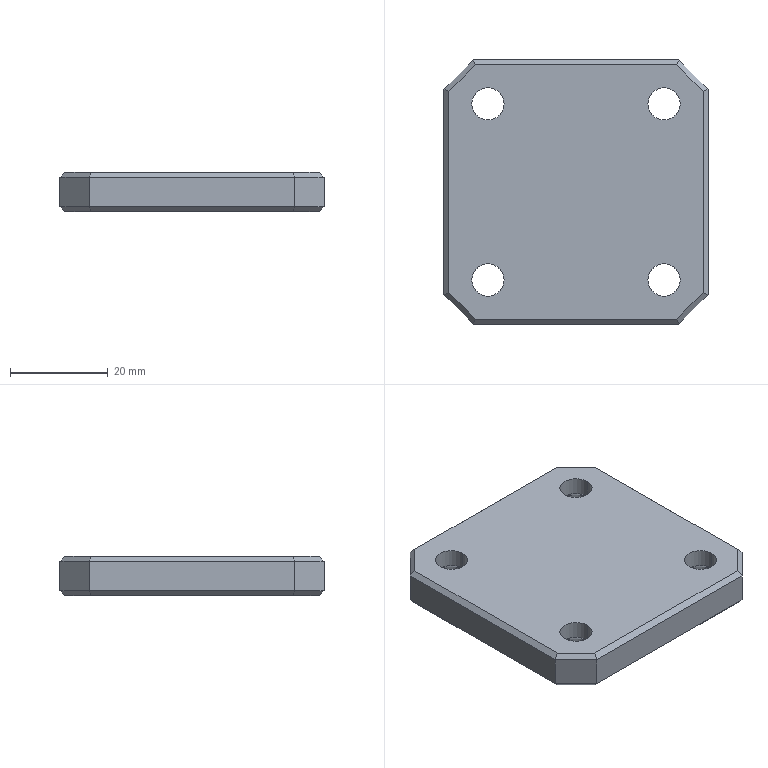Part | Creo | 1 solid | 50 faces | box 54 x 53.991 x 8 mm | volume 20318 mm3 | plane 26 | cylinder 16 | cone 8 | commonest cylinder face diameters 6.6 x8 13 x8
STEP:
#1=CARTESIAN_POINT('',(-106.,282.581,-2.));
#2=VERTEX_POINT('',#1);
#3=CARTESIAN_POINT('',(-106.,241.419,-2.));
#4=VERTEX_POINT('',#3);
#5=CARTESIAN_POINT('',(-106.,282.581,-2.));
#6=DIRECTION('',(0.,-1.,0.));
#7=VECTOR('',#6,41.162);
#8=LINE('',#5,#7);
#9=EDGE_CURVE('',#2,#4,#8,.T.);
#10=ORIENTED_EDGE('',*,*,#9,.T.);
#11=CARTESIAN_POINT('',(-111.414,236.005,-2.));
#12=VERTEX_POINT('',#11);
#13=CARTESIAN_POINT('',(-111.414,236.005,-2.));
#14=DIRECTION('',(0.7071,0.7071,0.));
#15=VECTOR('',#14,7.657);
#16=LINE('',#13,#15);
#17=EDGE_CURVE('',#12,#4,#16,.T.);
#18=ORIENTED_EDGE('',*,*,#17,.F.);
#19=CARTESIAN_POINT('',(-152.586,236.005,-2.));
#20=VERTEX_POINT('',#19);
#21=CARTESIAN_POINT('',(-111.414,236.005,-2.));
#22=DIRECTION('',(-1.,0.,0.));
#23=VECTOR('',#22,41.172);
#24=LINE('',#21,#23);
#25=EDGE_CURVE('',#12,#20,#24,.T.);
#26=ORIENTED_EDGE('',*,*,#25,.T.);
#27=CARTESIAN_POINT('',(-158.,241.419,-2.));
#28=VERTEX_POINT('',#27);
#29=CARTESIAN_POINT('',(-158.,241.419,-2.));
#30=DIRECTION('',(0.7071,-0.7071,0.));
#31=VECTOR('',#30,7.657);
#32=LINE('',#29,#31);
#33=EDGE_CURVE('',#28,#20,#32,.T.);
#34=ORIENTED_EDGE('',*,*,#33,.F.);
#35=CARTESIAN_POINT('',(-158.,282.581,-2.));
#36=VERTEX_POINT('',#35);
#37=CARTESIAN_POINT('',(-158.,241.419,-2.));
#38=DIRECTION('',(0.,1.,0.));
#39=VECTOR('',#38,41.162);
#40=LINE('',#37,#39);
#41=EDGE_CURVE('',#28,#36,#40,.T.);
#42=ORIENTED_EDGE('',*,*,#41,.T.);
#43=CARTESIAN_POINT('',(-152.586,287.995,-2.));
#44=VERTEX_POINT('',#43);
#45=CARTESIAN_POINT('',(-152.586,287.995,-2.));
#46=DIRECTION('',(-0.7071,-0.7071,0.));
#47=VECTOR('',#46,7.657);
#48=LINE('',#45,#47);
#49=EDGE_CURVE('',#44,#36,#48,.T.);
#50=ORIENTED_EDGE('',*,*,#49,.F.);
#51=CARTESIAN_POINT('',(-111.414,287.995,-2.));
#52=VERTEX_POINT('',#51);
#53=CARTESIAN_POINT('',(-152.586,287.995,-2.));
#54=DIRECTION('',(1.,0.,0.));
#55=VECTOR('',#54,41.172);
#56=LINE('',#53,#55);
#57=EDGE_CURVE('',#44,#52,#56,.T.);
#58=ORIENTED_EDGE('',*,*,#57,.T.);
#59=CARTESIAN_POINT('',(-106.,282.581,-2.));
#60=DIRECTION('',(-0.7071,0.7071,0.));
#61=VECTOR('',#60,7.657);
#62=LINE('',#59,#61);
#63=EDGE_CURVE('',#2,#52,#62,.T.);
#64=ORIENTED_EDGE('',*,*,#63,.F.);
#65=EDGE_LOOP('',(#10,#18,#26,#34,#42,#50,#58,#64));
#66=FACE_OUTER_BOUND('',#65,.F.);
#67=CARTESIAN_POINT('',(-110.7,280.005,-2.));
#68=VERTEX_POINT('',#67);
#69=CARTESIAN_POINT('',(-117.3,280.005,-2.));
#70=VERTEX_POINT('',#69);
#71=CARTESIAN_POINT('',(-114.,280.005,-2.));
#72=DIRECTION('',(0.,0.,-1.));
#73=DIRECTION('',(1.,0.,0.));
#74=AXIS2_PLACEMENT_3D('',#71,#72,#73);
#75=CIRCLE('',#74,3.3);
#76=EDGE_CURVE('',#68,#70,#75,.T.);
#77=ORIENTED_EDGE('',*,*,#76,.F.);
#78=CARTESIAN_POINT('',(-114.,280.005,-2.));
#79=DIRECTION('',(0.,0.,-1.));
#80=DIRECTION('',(-1.,0.,0.));
#81=AXIS2_PLACEMENT_3D('',#78,#79,#80);
#82=CIRCLE('',#81,3.3);
#83=EDGE_CURVE('',#70,#68,#82,.T.);
#84=ORIENTED_EDGE('',*,*,#83,.F.);
#85=EDGE_LOOP('',(#77,#84));
#86=FACE_BOUND('',#85,.F.);
#87=CARTESIAN_POINT('',(-146.7,280.005,-2.));
#88=VERTEX_POINT('',#87);
#89=CARTESIAN_POINT('',(-153.3,280.005,-2.));
#90=VERTEX_POINT('',#89);
#91=CARTESIAN_POINT('',(-150.,280.005,-2.));
#92=DIRECTION('',(0.,0.,-1.));
#93=DIRECTION('',(1.,0.,0.));
#94=AXIS2_PLACEMENT_3D('',#91,#92,#93);
#95=CIRCLE('',#94,3.3);
#96=EDGE_CURVE('',#88,#90,#95,.T.);
#97=ORIENTED_EDGE('',*,*,#96,.F.);
#98=CARTESIAN_POINT('',(-150.,280.005,-2.));
#99=DIRECTION('',(0.,0.,-1.));
#100=DIRECTION('',(-1.,0.,0.));
#101=AXIS2_PLACEMENT_3D('',#98,#99,#100);
#102=CIRCLE('',#101,3.3);
#103=EDGE_CURVE('',#90,#88,#102,.T.);
#104=ORIENTED_EDGE('',*,*,#103,.F.);
#105=EDGE_LOOP('',(#97,#104));
#106=FACE_BOUND('',#105,.F.);
#107=CARTESIAN_POINT('',(-110.7,244.005,-2.));
#108=VERTEX_POINT('',#107);
#109=CARTESIAN_POINT('',(-117.3,244.005,-2.));
#110=VERTEX_POINT('',#109);
#111=CARTESIAN_POINT('',(-114.,244.005,-2.));
#112=DIRECTION('',(0.,0.,-1.));
#113=DIRECTION('',(1.,0.,0.));
#114=AXIS2_PLACEMENT_3D('',#111,#112,#113);
#115=CIRCLE('',#114,3.3);
#116=EDGE_CURVE('',#108,#110,#115,.T.);
#117=ORIENTED_EDGE('',*,*,#116,.F.);
#118=CARTESIAN_POINT('',(-114.,244.005,-2.));
#119=DIRECTION('',(0.,0.,-1.));
#120=DIRECTION('',(-1.,0.,0.));
#121=AXIS2_PLACEMENT_3D('',#118,#119,#120);
#122=CIRCLE('',#121,3.3);
#123=EDGE_CURVE('',#110,#108,#122,.T.);
#124=ORIENTED_EDGE('',*,*,#123,.F.);
#125=EDGE_LOOP('',(#117,#124));
#126=FACE_BOUND('',#125,.F.);
#127=CARTESIAN_POINT('',(-146.7,244.005,-2.));
#128=VERTEX_POINT('',#127);
#129=CARTESIAN_POINT('',(-153.3,244.005,-2.));
#130=VERTEX_POINT('',#129);
#131=CARTESIAN_POINT('',(-150.,244.005,-2.));
#132=DIRECTION('',(0.,0.,-1.));
#133=DIRECTION('',(1.,0.,0.));
#134=AXIS2_PLACEMENT_3D('',#131,#132,#133);
#135=CIRCLE('',#134,3.3);
#136=EDGE_CURVE('',#128,#130,#135,.T.);
#137=ORIENTED_EDGE('',*,*,#136,.F.);
#138=CARTESIAN_POINT('',(-150.,244.005,-2.));
#139=DIRECTION('',(0.,0.,-1.));
#140=DIRECTION('',(-1.,0.,0.));
#141=AXIS2_PLACEMENT_3D('',#138,#139,#140);
#142=CIRCLE('',#141,3.3);
#143=EDGE_CURVE('',#130,#128,#142,.T.);
#144=ORIENTED_EDGE('',*,*,#143,.F.);
#145=EDGE_LOOP('',(#137,#144));
#146=FACE_BOUND('',#145,.F.);
#147=CARTESIAN_POINT('',(-132.,262.005,-2.));
#148=DIRECTION('',(0.,0.,1.));
#149=DIRECTION('',(-1.,0.,0.));
#150=AXIS2_PLACEMENT_3D('',#147,#148,#149);
#151=PLANE('',#150);
#152=ADVANCED_FACE('',(#66,#86,#106,#126,#146),#151,.T.);
#153=CARTESIAN_POINT('',(-105.,282.995,-3.));
#154=VERTEX_POINT('',#153);
#155=CARTESIAN_POINT('',(-106.,282.581,-2.));
#156=DIRECTION('',(0.6786,0.2811,-0.6786));
#157=VECTOR('',#156,1.474);
#158=LINE('',#155,#157);
#159=EDGE_CURVE('',#2,#154,#158,.T.);
#160=ORIENTED_EDGE('',*,*,#159,.T.);
#161=CARTESIAN_POINT('',(-105.,241.005,-3.));
#162=VERTEX_POINT('',#161);
#163=CARTESIAN_POINT('',(-105.,241.005,-3.));
#164=DIRECTION('',(0.,1.,0.));
#165=VECTOR('',#164,41.991);
#166=LINE('',#163,#165);
#167=EDGE_CURVE('',#162,#154,#166,.T.);
#168=ORIENTED_EDGE('',*,*,#167,.F.);
#169=CARTESIAN_POINT('',(-106.,241.419,-2.));
#170=DIRECTION('',(0.6786,-0.2811,-0.6786));
#171=VECTOR('',#170,1.474);
#172=LINE('',#169,#171);
#173=EDGE_CURVE('',#4,#162,#172,.T.);
#174=ORIENTED_EDGE('',*,*,#173,.F.);
#175=ORIENTED_EDGE('',*,*,#9,.F.);
#176=EDGE_LOOP('',(#160,#168,#174,#175));
#177=FACE_OUTER_BOUND('',#176,.F.);
#178=CARTESIAN_POINT('',(-105.,262.005,-3.));
#179=DIRECTION('',(-0.7071,0.,-0.7071));
#180=DIRECTION('',(0.,-1.,0.));
#181=AXIS2_PLACEMENT_3D('',#178,#179,#180);
#182=PLANE('',#181);
#183=ADVANCED_FACE('',(#177),#182,.F.);
#184=CARTESIAN_POINT('',(-111.,288.995,-3.));
#185=VERTEX_POINT('',#184);
#186=CARTESIAN_POINT('',(-111.414,287.995,-2.));
#187=DIRECTION('',(0.2811,0.6786,-0.6786));
#188=VECTOR('',#187,1.474);
#189=LINE('',#186,#188);
#190=EDGE_CURVE('',#52,#185,#189,.T.);
#191=ORIENTED_EDGE('',*,*,#190,.T.);
#192=CARTESIAN_POINT('',(-105.,282.995,-3.));
#193=DIRECTION('',(-0.7071,0.7071,0.));
#194=VECTOR('',#193,8.485);
#195=LINE('',#192,#194);
#196=EDGE_CURVE('',#154,#185,#195,.T.);
#197=ORIENTED_EDGE('',*,*,#196,.F.);
#198=ORIENTED_EDGE('',*,*,#159,.F.);
#199=ORIENTED_EDGE('',*,*,#63,.T.);
#200=EDGE_LOOP('',(#191,#197,#198,#199));
#201=FACE_OUTER_BOUND('',#200,.F.);
#202=CARTESIAN_POINT('',(-108.712,285.293,-2.));
#203=DIRECTION('',(0.5,0.5,0.7071));
#204=DIRECTION('',(0.7071,-0.7071,0.));
#205=AXIS2_PLACEMENT_3D('',#202,#203,#204);
#206=PLANE('',#205);
#207=ADVANCED_FACE('',(#201),#206,.T.);
#208=CARTESIAN_POINT('',(-153.,288.995,-3.));
#209=VERTEX_POINT('',#208);
#210=CARTESIAN_POINT('',(-153.,288.995,-3.));
#211=DIRECTION('',(0.2811,-0.6786,0.6786));
#212=VECTOR('',#211,1.474);
#213=LINE('',#210,#212);
#214=EDGE_CURVE('',#209,#44,#213,.T.);
#215=ORIENTED_EDGE('',*,*,#214,.F.);
#216=CARTESIAN_POINT('',(-111.,288.995,-3.));
#217=DIRECTION('',(-1.,0.,0.));
#218=VECTOR('',#217,42.);
#219=LINE('',#216,#218);
#220=EDGE_CURVE('',#185,#209,#219,.T.);
#221=ORIENTED_EDGE('',*,*,#220,.F.);
#222=ORIENTED_EDGE('',*,*,#190,.F.);
#223=ORIENTED_EDGE('',*,*,#57,.F.);
#224=EDGE_LOOP('',(#215,#221,#222,#223));
#225=FACE_OUTER_BOUND('',#224,.F.);
#226=CARTESIAN_POINT('',(-132.,288.995,-3.));
#227=DIRECTION('',(0.,-0.7071,-0.7071));
#228=DIRECTION('',(1.,0.,0.));
#229=AXIS2_PLACEMENT_3D('',#226,#227,#228);
#230=PLANE('',#229);
#231=ADVANCED_FACE('',(#225),#230,.F.);
#232=ORIENTED_EDGE('',*,*,#214,.T.);
#233=ORIENTED_EDGE('',*,*,#49,.T.);
#234=CARTESIAN_POINT('',(-159.,282.995,-3.));
#235=VERTEX_POINT('',#234);
#236=CARTESIAN_POINT('',(-159.,282.995,-3.));
#237=DIRECTION('',(0.6786,-0.2811,0.6786));
#238=VECTOR('',#237,1.474);
#239=LINE('',#236,#238);
#240=EDGE_CURVE('',#235,#36,#239,.T.);
#241=ORIENTED_EDGE('',*,*,#240,.F.);
#242=CARTESIAN_POINT('',(-153.,288.995,-3.));
#243=DIRECTION('',(-0.7071,-0.7071,0.));
#244=VECTOR('',#243,8.485);
#245=LINE('',#242,#244);
#246=EDGE_CURVE('',#209,#235,#245,.T.);
#247=ORIENTED_EDGE('',*,*,#246,.F.);
#248=EDGE_LOOP('',(#232,#233,#241,#247));
#249=FACE_OUTER_BOUND('',#248,.F.);
#250=CARTESIAN_POINT('',(-155.288,285.293,-2.));
#251=DIRECTION('',(-0.5,0.5,0.7071));
#252=DIRECTION('',(0.7071,0.7071,0.));
#253=AXIS2_PLACEMENT_3D('',#250,#251,#252);
#254=PLANE('',#253);
#255=ADVANCED_FACE('',(#249),#254,.T.);
#256=ORIENTED_EDGE('',*,*,#240,.T.);
#257=ORIENTED_EDGE('',*,*,#41,.F.);
#258=CARTESIAN_POINT('',(-159.,241.005,-3.));
#259=VERTEX_POINT('',#258);
#260=CARTESIAN_POINT('',(-159.,241.005,-3.));
#261=DIRECTION('',(0.6786,0.2811,0.6786));
#262=VECTOR('',#261,1.474);
#263=LINE('',#260,#262);
#264=EDGE_CURVE('',#259,#28,#263,.T.);
#265=ORIENTED_EDGE('',*,*,#264,.F.);
#266=CARTESIAN_POINT('',(-159.,282.995,-3.));
#267=DIRECTION('',(0.,-1.,0.));
#268=VECTOR('',#267,41.991);
#269=LINE('',#266,#268);
#270=EDGE_CURVE('',#235,#259,#269,.T.);
#271=ORIENTED_EDGE('',*,*,#270,.F.);
#272=EDGE_LOOP('',(#256,#257,#265,#271));
#273=FACE_OUTER_BOUND('',#272,.F.);
#274=CARTESIAN_POINT('',(-159.,262.005,-3.));
#275=DIRECTION('',(0.7071,0.,-0.7071));
#276=DIRECTION('',(0.,1.,0.));
#277=AXIS2_PLACEMENT_3D('',#274,#275,#276);
#278=PLANE('',#277);
#279=ADVANCED_FACE('',(#273),#278,.F.);
#280=ORIENTED_EDGE('',*,*,#264,.T.);
#281=ORIENTED_EDGE('',*,*,#33,.T.);
#282=CARTESIAN_POINT('',(-153.,235.005,-3.));
#283=VERTEX_POINT('',#282);
#284=CARTESIAN_POINT('',(-153.,235.005,-3.));
#285=DIRECTION('',(0.2811,0.6786,0.6786));
#286=VECTOR('',#285,1.474);
#287=LINE('',#284,#286);
#288=EDGE_CURVE('',#283,#20,#287,.T.);
#289=ORIENTED_EDGE('',*,*,#288,.F.);
#290=CARTESIAN_POINT('',(-159.,241.005,-3.));
#291=DIRECTION('',(0.7071,-0.7071,0.));
#292=VECTOR('',#291,8.485);
#293=LINE('',#290,#292);
#294=EDGE_CURVE('',#259,#283,#293,.T.);
#295=ORIENTED_EDGE('',*,*,#294,.F.);
#296=EDGE_LOOP('',(#280,#281,#289,#295));
#297=FACE_OUTER_BOUND('',#296,.F.);
#298=CARTESIAN_POINT('',(-155.293,238.712,-2.));
#299=DIRECTION('',(-0.5,-0.5,0.7071));
#300=DIRECTION('',(-0.7071,0.7071,0.));
#301=AXIS2_PLACEMENT_3D('',#298,#299,#300);
#302=PLANE('',#301);
#303=ADVANCED_FACE('',(#297),#302,.T.);
#304=CARTESIAN_POINT('',(-111.,235.005,-3.));
#305=VERTEX_POINT('',#304);
#306=CARTESIAN_POINT('',(-111.414,236.005,-2.));
#307=DIRECTION('',(0.2811,-0.6786,-0.6786));
#308=VECTOR('',#307,1.474);
#309=LINE('',#306,#308);
#310=EDGE_CURVE('',#12,#305,#309,.T.);
#311=ORIENTED_EDGE('',*,*,#310,.T.);
#312=CARTESIAN_POINT('',(-153.,235.005,-3.));
#313=DIRECTION('',(1.,0.,0.));
#314=VECTOR('',#313,42.);
#315=LINE('',#312,#314);
#316=EDGE_CURVE('',#283,#305,#315,.T.);
#317=ORIENTED_EDGE('',*,*,#316,.F.);
#318=ORIENTED_EDGE('',*,*,#288,.T.);
#319=ORIENTED_EDGE('',*,*,#25,.F.);
#320=EDGE_LOOP('',(#311,#317,#318,#319));
#321=FACE_OUTER_BOUND('',#320,.F.);
#322=CARTESIAN_POINT('',(-132.,235.005,-3.));
#323=DIRECTION('',(0.,0.7071,-0.7071));
#324=DIRECTION('',(-1.,0.,0.));
#325=AXIS2_PLACEMENT_3D('',#322,#323,#324);
#326=PLANE('',#325);
#327=ADVANCED_FACE('',(#321),#326,.F.);
#328=ORIENTED_EDGE('',*,*,#173,.T.);
#329=CARTESIAN_POINT('',(-111.,235.005,-3.));
#330=DIRECTION('',(0.7071,0.7071,0.));
#331=VECTOR('',#330,8.485);
#332=LINE('',#329,#331);
#333=EDGE_CURVE('',#305,#162,#332,.T.);
#334=ORIENTED_EDGE('',*,*,#333,.F.);
#335=ORIENTED_EDGE('',*,*,#310,.F.);
#336=ORIENTED_EDGE('',*,*,#17,.T.);
#337=EDGE_LOOP('',(#328,#334,#335,#336));
#338=FACE_OUTER_BOUND('',#337,.F.);
#339=CARTESIAN_POINT('',(-108.707,238.712,-2.));
#340=DIRECTION('',(0.5,-0.5,0.7071));
#341=DIRECTION('',(-0.7071,-0.7071,0.));
#342=AXIS2_PLACEMENT_3D('',#339,#340,#341);
#343=PLANE('',#342);
#344=ADVANCED_FACE('',(#338),#343,.T.);
#345=CARTESIAN_POINT('',(-105.,241.005,-9.));
#346=VERTEX_POINT('',#345);
#347=CARTESIAN_POINT('',(-105.,241.005,-9.));
#348=DIRECTION('',(0.,0.,1.));
#349=VECTOR('',#348,6.);
#350=LINE('',#347,#349);
#351=EDGE_CURVE('',#346,#162,#350,.T.);
#352=ORIENTED_EDGE('',*,*,#351,.F.);
#353=CARTESIAN_POINT('',(-111.,235.005,-9.));
#354=VERTEX_POINT('',#353);
#355=CARTESIAN_POINT('',(-105.,241.005,-9.));
#356=DIRECTION('',(-0.7071,-0.7071,0.));
#357=VECTOR('',#356,8.485);
#358=LINE('',#355,#357);
#359=EDGE_CURVE('',#346,#354,#358,.T.);
#360=ORIENTED_EDGE('',*,*,#359,.T.);
#361=CARTESIAN_POINT('',(-111.,235.005,-3.));
#362=DIRECTION('',(0.,0.,-1.));
#363=VECTOR('',#362,6.);
#364=LINE('',#361,#363);
#365=EDGE_CURVE('',#305,#354,#364,.T.);
#366=ORIENTED_EDGE('',*,*,#365,.F.);
#367=ORIENTED_EDGE('',*,*,#333,.T.);
#368=EDGE_LOOP('',(#352,#360,#366,#367));
#369=FACE_OUTER_BOUND('',#368,.F.);
#370=CARTESIAN_POINT('',(-105.,241.005,-11.));
#371=DIRECTION('',(-0.7071,0.7071,0.));
#372=DIRECTION('',(0.,0.,-1.));
#373=AXIS2_PLACEMENT_3D('',#370,#371,#372);
#374=PLANE('',#373);
#375=ADVANCED_FACE('',(#369),#374,.F.);
#376=ORIENTED_EDGE('',*,*,#351,.T.);
#377=ORIENTED_EDGE('',*,*,#167,.T.);
#378=CARTESIAN_POINT('',(-105.,282.995,-9.));
#379=VERTEX_POINT('',#378);
#380=CARTESIAN_POINT('',(-105.,282.995,-3.));
#381=DIRECTION('',(0.,0.,-1.));
#382=VECTOR('',#381,6.);
#383=LINE('',#380,#382);
#384=EDGE_CURVE('',#154,#379,#383,.T.);
#385=ORIENTED_EDGE('',*,*,#384,.T.);
#386=CARTESIAN_POINT('',(-105.,282.995,-9.));
#387=DIRECTION('',(0.,-1.,0.));
#388=VECTOR('',#387,41.991);
#389=LINE('',#386,#388);
#390=EDGE_CURVE('',#379,#346,#389,.T.);
#391=ORIENTED_EDGE('',*,*,#390,.T.);
#392=EDGE_LOOP('',(#376,#377,#385,#391));
#393=FACE_OUTER_BOUND('',#392,.F.);
#394=CARTESIAN_POINT('',(-105.,262.005,-11.));
#395=DIRECTION('',(1.,0.,0.));
#396=DIRECTION('',(0.,0.,1.));
#397=AXIS2_PLACEMENT_3D('',#394,#395,#396);
#398=PLANE('',#397);
#399=ADVANCED_FACE('',(#393),#398,.T.);
#400=CARTESIAN_POINT('',(-111.,288.995,-9.));
#401=VERTEX_POINT('',#400);
#402=CARTESIAN_POINT('',(-111.,288.995,-9.));
#403=DIRECTION('',(0.,0.,1.));
#404=VECTOR('',#403,6.);
#405=LINE('',#402,#404);
#406=EDGE_CURVE('',#401,#185,#405,.T.);
#407=ORIENTED_EDGE('',*,*,#406,.F.);
#408=CARTESIAN_POINT('',(-111.,288.995,-9.));
#409=DIRECTION('',(0.7071,-0.7071,0.));
#410=VECTOR('',#409,8.485);
#411=LINE('',#408,#410);
#412=EDGE_CURVE('',#401,#379,#411,.T.);
#413=ORIENTED_EDGE('',*,*,#412,.T.);
#414=ORIENTED_EDGE('',*,*,#384,.F.);
#415=ORIENTED_EDGE('',*,*,#196,.T.);
#416=EDGE_LOOP('',(#407,#413,#414,#415));
#417=FACE_OUTER_BOUND('',#416,.F.);
#418=CARTESIAN_POINT('',(-111.,288.995,-10.));
#419=DIRECTION('',(-0.7071,-0.7071,0.));
#420=DIRECTION('',(0.,0.,-1.));
#421=AXIS2_PLACEMENT_3D('',#418,#419,#420);
#422=PLANE('',#421);
#423=ADVANCED_FACE('',(#417),#422,.F.);
#424=CARTESIAN_POINT('',(-153.,288.995,-9.));
#425=VERTEX_POINT('',#424);
#426=CARTESIAN_POINT('',(-153.,288.995,-3.));
#427=DIRECTION('',(0.,0.,-1.));
#428=VECTOR('',#427,6.);
#429=LINE('',#426,#428);
#430=EDGE_CURVE('',#209,#425,#429,.T.);
#431=ORIENTED_EDGE('',*,*,#430,.T.);
#432=CARTESIAN_POINT('',(-153.,288.995,-9.));
#433=DIRECTION('',(1.,0.,0.));
#434=VECTOR('',#433,42.);
#435=LINE('',#432,#434);
#436=EDGE_CURVE('',#425,#401,#435,.T.);
#437=ORIENTED_EDGE('',*,*,#436,.T.);
#438=ORIENTED_EDGE('',*,*,#406,.T.);
#439=ORIENTED_EDGE('',*,*,#220,.T.);
#440=EDGE_LOOP('',(#431,#437,#438,#439));
#441=FACE_OUTER_BOUND('',#440,.F.);
#442=CARTESIAN_POINT('',(-132.,288.995,-10.));
#443=DIRECTION('',(0.,1.,0.));
#444=DIRECTION('',(0.,0.,1.));
#445=AXIS2_PLACEMENT_3D('',#442,#443,#444);
#446=PLANE('',#445);
#447=ADVANCED_FACE('',(#441),#446,.T.);
#448=CARTESIAN_POINT('',(-159.,282.995,-9.));
#449=VERTEX_POINT('',#448);
#450=CARTESIAN_POINT('',(-159.,282.995,-9.));
#451=DIRECTION('',(0.,0.,1.));
#452=VECTOR('',#451,6.);
#453=LINE('',#450,#452);
#454=EDGE_CURVE('',#449,#235,#453,.T.);
#455=ORIENTED_EDGE('',*,*,#454,.F.);
#456=CARTESIAN_POINT('',(-159.,282.995,-9.));
#457=DIRECTION('',(0.7071,0.7071,0.));
#458=VECTOR('',#457,8.485);
#459=LINE('',#456,#458);
#460=EDGE_CURVE('',#449,#425,#459,.T.);
#461=ORIENTED_EDGE('',*,*,#460,.T.);
#462=ORIENTED_EDGE('',*,*,#430,.F.);
#463=ORIENTED_EDGE('',*,*,#246,.T.);
#464=EDGE_LOOP('',(#455,#461,#462,#463));
#465=FACE_OUTER_BOUND('',#464,.F.);
#466=CARTESIAN_POINT('',(-153.,288.995,-10.));
#467=DIRECTION('',(0.7071,-0.7071,0.));
#468=DIRECTION('',(0.,0.,1.));
#469=AXIS2_PLACEMENT_3D('',#466,#467,#468);
#470=PLANE('',#469);
#471=ADVANCED_FACE('',(#465),#470,.F.);
#472=ORIENTED_EDGE('',*,*,#454,.T.);
#473=ORIENTED_EDGE('',*,*,#270,.T.);
#474=CARTESIAN_POINT('',(-159.,241.005,-9.));
#475=VERTEX_POINT('',#474);
#476=CARTESIAN_POINT('',(-159.,241.005,-3.));
#477=DIRECTION('',(0.,0.,-1.));
#478=VECTOR('',#477,6.);
#479=LINE('',#476,#478);
#480=EDGE_CURVE('',#259,#475,#479,.T.);
#481=ORIENTED_EDGE('',*,*,#480,.T.);
#482=CARTESIAN_POINT('',(-159.,241.005,-9.));
#483=DIRECTION('',(0.,1.,0.));
#484=VECTOR('',#483,41.991);
#485=LINE('',#482,#484);
#486=EDGE_CURVE('',#475,#449,#485,.T.);
#487=ORIENTED_EDGE('',*,*,#486,.T.);
#488=EDGE_LOOP('',(#472,#473,#481,#487));
#489=FACE_OUTER_BOUND('',#488,.F.);
#490=CARTESIAN_POINT('',(-159.,262.005,-11.));
#491=DIRECTION('',(-1.,0.,0.));
#492=DIRECTION('',(0.,0.,-1.));
#493=AXIS2_PLACEMENT_3D('',#490,#491,#492);
#494=PLANE('',#493);
#495=ADVANCED_FACE('',(#489),#494,.T.);
#496=CARTESIAN_POINT('',(-153.,235.005,-9.));
#497=VERTEX_POINT('',#496);
#498=CARTESIAN_POINT('',(-153.,235.005,-9.));
#499=DIRECTION('',(0.,0.,1.));
#500=VECTOR('',#499,6.);
#501=LINE('',#498,#500);
#502=EDGE_CURVE('',#497,#283,#501,.T.);
#503=ORIENTED_EDGE('',*,*,#502,.F.);
#504=CARTESIAN_POINT('',(-153.,235.005,-9.));
#505=DIRECTION('',(-0.7071,0.7071,0.));
#506=VECTOR('',#505,8.485);
#507=LINE('',#504,#506);
#508=EDGE_CURVE('',#497,#475,#507,.T.);
#509=ORIENTED_EDGE('',*,*,#508,.T.);
#510=ORIENTED_EDGE('',*,*,#480,.F.);
#511=ORIENTED_EDGE('',*,*,#294,.T.);
#512=EDGE_LOOP('',(#503,#509,#510,#511));
#513=FACE_OUTER_BOUND('',#512,.F.);
#514=CARTESIAN_POINT('',(-159.,241.005,-11.));
#515=DIRECTION('',(0.7071,0.7071,0.));
#516=DIRECTION('',(0.,0.,1.));
#517=AXIS2_PLACEMENT_3D('',#514,#515,#516);
#518=PLANE('',#517);
#519=ADVANCED_FACE('',(#513),#518,.F.);
#520=ORIENTED_EDGE('',*,*,#502,.T.);
#521=ORIENTED_EDGE('',*,*,#316,.T.);
#522=ORIENTED_EDGE('',*,*,#365,.T.);
#523=CARTESIAN_POINT('',(-111.,235.005,-9.));
#524=DIRECTION('',(-1.,0.,0.));
#525=VECTOR('',#524,42.);
#526=LINE('',#523,#525);
#527=EDGE_CURVE('',#354,#497,#526,.T.);
#528=ORIENTED_EDGE('',*,*,#527,.T.);
#529=EDGE_LOOP('',(#520,#521,#522,#528));
#530=FACE_OUTER_BOUND('',#529,.F.);
#531=CARTESIAN_POINT('',(-132.,235.005,-11.));
#532=DIRECTION('',(0.,-1.,0.));
#533=DIRECTION('',(0.,0.,1.));
#534=AXIS2_PLACEMENT_3D('',#531,#532,#533);
#535=PLANE('',#534);
#536=ADVANCED_FACE('',(#530),#535,.T.);
#537=CARTESIAN_POINT('',(-152.586,236.005,-10.));
#538=VERTEX_POINT('',#537);
#539=CARTESIAN_POINT('',(-152.586,236.005,-10.));
#540=DIRECTION('',(-0.2811,-0.6786,0.6786));
#541=VECTOR('',#540,1.474);
#542=LINE('',#539,#541);
#543=EDGE_CURVE('',#538,#497,#542,.T.);
#544=ORIENTED_EDGE('',*,*,#543,.T.);
#545=ORIENTED_EDGE('',*,*,#527,.F.);
#546=CARTESIAN_POINT('',(-111.414,236.005,-10.));
#547=VERTEX_POINT('',#546);
#548=CARTESIAN_POINT('',(-111.,235.005,-9.));
#549=DIRECTION('',(-0.2811,0.6786,-0.6786));
#550=VECTOR('',#549,1.474);
#551=LINE('',#548,#550);
#552=EDGE_CURVE('',#354,#547,#551,.T.);
#553=ORIENTED_EDGE('',*,*,#552,.T.);
#554=CARTESIAN_POINT('',(-152.586,236.005,-10.));
#555=DIRECTION('',(1.,0.,0.));
#556=VECTOR('',#555,41.172);
#557=LINE('',#554,#556);
#558=EDGE_CURVE('',#538,#547,#557,.T.);
#559=ORIENTED_EDGE('',*,*,#558,.F.);
#560=EDGE_LOOP('',(#544,#545,#553,#559));
#561=FACE_OUTER_BOUND('',#560,.F.);
#562=CARTESIAN_POINT('',(-132.,235.005,-9.));
#563=DIRECTION('',(0.,0.7071,0.7071));
#564=DIRECTION('',(1.,0.,0.));
#565=AXIS2_PLACEMENT_3D('',#562,#563,#564);
#566=PLANE('',#565);
#567=ADVANCED_FACE('',(#561),#566,.F.);
#568=CARTESIAN_POINT('',(-158.,241.419,-10.));
#569=VERTEX_POINT('',#568);
#570=CARTESIAN_POINT('',(-158.,241.419,-10.));
#571=DIRECTION('',(-0.6786,-0.2811,0.6786));
#572=VECTOR('',#571,1.474);
#573=LINE('',#570,#572);
#574=EDGE_CURVE('',#569,#475,#573,.T.);
#575=ORIENTED_EDGE('',*,*,#574,.T.);
#576=ORIENTED_EDGE('',*,*,#508,.F.);
#577=ORIENTED_EDGE('',*,*,#543,.F.);
#578=CARTESIAN_POINT('',(-152.586,236.005,-10.));
#579=DIRECTION('',(-0.7071,0.7071,0.));
#580=VECTOR('',#579,7.657);
#581=LINE('',#578,#580);
#582=EDGE_CURVE('',#538,#569,#581,.T.);
#583=ORIENTED_EDGE('',*,*,#582,.T.);
#584=EDGE_LOOP('',(#575,#576,#577,#583));
#585=FACE_OUTER_BOUND('',#584,.F.);
#586=CARTESIAN_POINT('',(120.707,-37.288,-10.));
#587=DIRECTION('',(-0.5,-0.5,-0.7071));
#588=DIRECTION('',(0.7071,-0.7071,0.));
#589=AXIS2_PLACEMENT_3D('',#586,#587,#588);
#590=PLANE('',#589);
#591=ADVANCED_FACE('',(#585),#590,.T.);
#592=CARTESIAN_POINT('',(-158.,282.581,-10.));
#593=VERTEX_POINT('',#592);
#594=CARTESIAN_POINT('',(-158.,282.581,-10.));
#595=DIRECTION('',(-0.6786,0.2811,0.6786));
#596=VECTOR('',#595,1.474);
#597=LINE('',#594,#596);
#598=EDGE_CURVE('',#593,#449,#597,.T.);
#599=ORIENTED_EDGE('',*,*,#598,.T.);
#600=ORIENTED_EDGE('',*,*,#486,.F.);
#601=ORIENTED_EDGE('',*,*,#574,.F.);
#602=CARTESIAN_POINT('',(-158.,282.581,-10.));
#603=DIRECTION('',(0.,-1.,0.));
#604=VECTOR('',#603,41.162);
#605=LINE('',#602,#604);
#606=EDGE_CURVE('',#593,#569,#605,.T.);
#607=ORIENTED_EDGE('',*,*,#606,.F.);
#608=EDGE_LOOP('',(#599,#600,#601,#607));
#609=FACE_OUTER_BOUND('',#608,.F.);
#610=CARTESIAN_POINT('',(-159.,262.005,-9.));
#611=DIRECTION('',(0.7071,0.,0.7071));
#612=DIRECTION('',(0.,-1.,0.));
#613=AXIS2_PLACEMENT_3D('',#610,#611,#612);
#614=PLANE('',#613);
#615=ADVANCED_FACE('',(#609),#614,.F.);
#616=CARTESIAN_POINT('',(-152.586,287.995,-10.));
#617=VERTEX_POINT('',#616);
#618=CARTESIAN_POINT('',(-152.586,287.995,-10.));
#619=DIRECTION('',(-0.2811,0.6786,0.6786));
#620=VECTOR('',#619,1.474);
#621=LINE('',#618,#620);
#622=EDGE_CURVE('',#617,#425,#621,.T.);
#623=ORIENTED_EDGE('',*,*,#622,.T.);
#624=ORIENTED_EDGE('',*,*,#460,.F.);
#625=ORIENTED_EDGE('',*,*,#598,.F.);
#626=CARTESIAN_POINT('',(-158.,282.581,-10.));
#627=DIRECTION('',(0.7071,0.7071,0.));
#628=VECTOR('',#627,7.657);
#629=LINE('',#626,#628);
#630=EDGE_CURVE('',#593,#617,#629,.T.);
#631=ORIENTED_EDGE('',*,*,#630,.T.);
#632=EDGE_LOOP('',(#623,#624,#625,#631));
#633=FACE_OUTER_BOUND('',#632,.F.);
#634=CARTESIAN_POINT('',(-141.288,299.293,-10.));
#635=DIRECTION('',(-0.5,0.5,-0.7071));
#636=DIRECTION('',(-0.7071,-0.7071,0.));
#637=AXIS2_PLACEMENT_3D('',#634,#635,#636);
#638=PLANE('',#637);
#639=ADVANCED_FACE('',(#633),#638,.T.);
#640=CARTESIAN_POINT('',(-111.414,287.995,-10.));
#641=VERTEX_POINT('',#640);
#642=CARTESIAN_POINT('',(-111.,288.995,-9.));
#643=DIRECTION('',(-0.2811,-0.6786,-0.6786));
#644=VECTOR('',#643,1.474);
#645=LINE('',#642,#644);
#646=EDGE_CURVE('',#401,#641,#645,.T.);
#647=ORIENTED_EDGE('',*,*,#646,.F.);
#648=ORIENTED_EDGE('',*,*,#436,.F.);
#649=ORIENTED_EDGE('',*,*,#622,.F.);
#650=CARTESIAN_POINT('',(-111.414,287.995,-10.));
#651=DIRECTION('',(-1.,0.,0.));
#652=VECTOR('',#651,41.172);
#653=LINE('',#650,#652);
#654=EDGE_CURVE('',#641,#617,#653,.T.);
#655=ORIENTED_EDGE('',*,*,#654,.F.);
#656=EDGE_LOOP('',(#647,#648,#649,#655));
#657=FACE_OUTER_BOUND('',#656,.F.);
#658=CARTESIAN_POINT('',(-132.,288.995,-9.));
#659=DIRECTION('',(0.,-0.7071,0.7071));
#660=DIRECTION('',(-1.,0.,0.));
#661=AXIS2_PLACEMENT_3D('',#658,#659,#660);
#662=PLANE('',#661);
#663=ADVANCED_FACE('',(#657),#662,.F.);
#664=ORIENTED_EDGE('',*,*,#646,.T.);
#665=CARTESIAN_POINT('',(-106.,282.581,-10.));
#666=VERTEX_POINT('',#665);
#667=CARTESIAN_POINT('',(-111.414,287.995,-10.));
#668=DIRECTION('',(0.7071,-0.7071,0.));
#669=VECTOR('',#668,7.657);
#670=LINE('',#667,#669);
#671=EDGE_CURVE('',#641,#666,#670,.T.);
#672=ORIENTED_EDGE('',*,*,#671,.T.);
#673=CARTESIAN_POINT('',(-105.,282.995,-9.));
#674=DIRECTION('',(-0.6786,-0.2811,-0.6786));
#675=VECTOR('',#674,1.474);
#676=LINE('',#673,#675);
#677=EDGE_CURVE('',#379,#666,#676,.T.);
#678=ORIENTED_EDGE('',*,*,#677,.F.);
#679=ORIENTED_EDGE('',*,*,#412,.F.);
#680=EDGE_LOOP('',(#664,#672,#678,#679));
#681=FACE_OUTER_BOUND('',#680,.F.);
#682=CARTESIAN_POINT('',(167.288,9.293,-10.));
#683=DIRECTION('',(0.5,0.5,-0.7071));
#684=DIRECTION('',(-0.7071,0.7071,0.));
#685=AXIS2_PLACEMENT_3D('',#682,#683,#684);
#686=PLANE('',#685);
#687=ADVANCED_FACE('',(#681),#686,.T.);
#688=ORIENTED_EDGE('',*,*,#654,.T.);
#689=ORIENTED_EDGE('',*,*,#630,.F.);
#690=ORIENTED_EDGE('',*,*,#606,.T.);
#691=ORIENTED_EDGE('',*,*,#582,.F.);
#692=ORIENTED_EDGE('',*,*,#558,.T.);
#693=CARTESIAN_POINT('',(-106.,241.419,-10.));
#694=VERTEX_POINT('',#693);
#695=CARTESIAN_POINT('',(-106.,241.419,-10.));
#696=DIRECTION('',(-0.7071,-0.7071,0.));
#697=VECTOR('',#696,7.657);
#698=LINE('',#695,#697);
#699=EDGE_CURVE('',#694,#547,#698,.T.);
#700=ORIENTED_EDGE('',*,*,#699,.F.);
#701=CARTESIAN_POINT('',(-106.,241.419,-10.));
#702=DIRECTION('',(0.,1.,0.));
#703=VECTOR('',#702,41.162);
#704=LINE('',#701,#703);
#705=EDGE_CURVE('',#694,#666,#704,.T.);
#706=ORIENTED_EDGE('',*,*,#705,.T.);
#707=ORIENTED_EDGE('',*,*,#671,.F.);
#708=EDGE_LOOP('',(#688,#689,#690,#691,#692,#700,#706,#707));
#709=FACE_OUTER_BOUND('',#708,.F.);
#710=CARTESIAN_POINT('',(-143.5,244.005,-10.));
#711=VERTEX_POINT('',#710);
#712=CARTESIAN_POINT('',(-156.5,244.005,-10.));
#713=VERTEX_POINT('',#712);
#714=CARTESIAN_POINT('',(-150.,244.005,-10.));
#715=DIRECTION('',(0.,0.,1.));
#716=DIRECTION('',(1.,0.,0.));
#717=AXIS2_PLACEMENT_3D('',#714,#715,#716);
#718=CIRCLE('',#717,6.5);
#719=EDGE_CURVE('',#711,#713,#718,.T.);
#720=ORIENTED_EDGE('',*,*,#719,.F.);
#721=CARTESIAN_POINT('',(-150.,244.005,-10.));
#722=DIRECTION('',(0.,0.,1.));
#723=DIRECTION('',(-1.,0.,0.));
#724=AXIS2_PLACEMENT_3D('',#721,#722,#723);
#725=CIRCLE('',#724,6.5);
#726=EDGE_CURVE('',#713,#711,#725,.T.);
#727=ORIENTED_EDGE('',*,*,#726,.F.);
#728=EDGE_LOOP('',(#720,#727));
#729=FACE_BOUND('',#728,.F.);
#730=CARTESIAN_POINT('',(-107.5,244.005,-10.));
#731=VERTEX_POINT('',#730);
#732=CARTESIAN_POINT('',(-120.5,244.005,-10.));
#733=VERTEX_POINT('',#732);
#734=CARTESIAN_POINT('',(-114.,244.005,-10.));
#735=DIRECTION('',(0.,0.,1.));
#736=DIRECTION('',(1.,0.,0.));
#737=AXIS2_PLACEMENT_3D('',#734,#735,#736);
#738=CIRCLE('',#737,6.5);
#739=EDGE_CURVE('',#731,#733,#738,.T.);
#740=ORIENTED_EDGE('',*,*,#739,.F.);
#741=CARTESIAN_POINT('',(-114.,244.005,-10.));
#742=DIRECTION('',(0.,0.,1.));
#743=DIRECTION('',(-1.,0.,0.));
#744=AXIS2_PLACEMENT_3D('',#741,#742,#743);
#745=CIRCLE('',#744,6.5);
#746=EDGE_CURVE('',#733,#731,#745,.T.);
#747=ORIENTED_EDGE('',*,*,#746,.F.);
#748=EDGE_LOOP('',(#740,#747));
#749=FACE_BOUND('',#748,.F.);
#750=CARTESIAN_POINT('',(-143.5,280.005,-10.));
#751=VERTEX_POINT('',#750);
#752=CARTESIAN_POINT('',(-156.5,280.005,-10.));
#753=VERTEX_POINT('',#752);
#754=CARTESIAN_POINT('',(-150.,280.005,-10.));
#755=DIRECTION('',(0.,0.,1.));
#756=DIRECTION('',(1.,0.,0.));
#757=AXIS2_PLACEMENT_3D('',#754,#755,#756);
#758=CIRCLE('',#757,6.5);
#759=EDGE_CURVE('',#751,#753,#758,.T.);
#760=ORIENTED_EDGE('',*,*,#759,.F.);
#761=CARTESIAN_POINT('',(-150.,280.005,-10.));
#762=DIRECTION('',(0.,0.,1.));
#763=DIRECTION('',(-1.,0.,0.));
#764=AXIS2_PLACEMENT_3D('',#761,#762,#763);
#765=CIRCLE('',#764,6.5);
#766=EDGE_CURVE('',#753,#751,#765,.T.);
#767=ORIENTED_EDGE('',*,*,#766,.F.);
#768=EDGE_LOOP('',(#760,#767));
#769=FACE_BOUND('',#768,.F.);
#770=CARTESIAN_POINT('',(-107.5,280.005,-10.));
#771=VERTEX_POINT('',#770);
#772=CARTESIAN_POINT('',(-120.5,280.005,-10.));
#773=VERTEX_POINT('',#772);
#774=CARTESIAN_POINT('',(-114.,280.005,-10.));
#775=DIRECTION('',(0.,0.,1.));
#776=DIRECTION('',(1.,0.,0.));
#777=AXIS2_PLACEMENT_3D('',#774,#775,#776);
#778=CIRCLE('',#777,6.5);
#779=EDGE_CURVE('',#771,#773,#778,.T.);
#780=ORIENTED_EDGE('',*,*,#779,.F.);
#781=CARTESIAN_POINT('',(-114.,280.005,-10.));
#782=DIRECTION('',(0.,0.,1.));
#783=DIRECTION('',(-1.,0.,0.));
#784=AXIS2_PLACEMENT_3D('',#781,#782,#783);
#785=CIRCLE('',#784,6.5);
#786=EDGE_CURVE('',#773,#771,#785,.T.);
#787=ORIENTED_EDGE('',*,*,#786,.F.);
#788=EDGE_LOOP('',(#780,#787));
#789=FACE_BOUND('',#788,.F.);
#790=CARTESIAN_POINT('',(158.,0.004699,-10.));
#791=DIRECTION('',(0.,0.,-1.));
#792=DIRECTION('',(1.,0.,0.));
#793=AXIS2_PLACEMENT_3D('',#790,#791,#792);
#794=PLANE('',#793);
#795=ADVANCED_FACE('',(#709,#729,#749,#769,#789),#794,.T.);
#796=CARTESIAN_POINT('',(-105.,241.005,-9.));
#797=DIRECTION('',(-0.6786,0.2811,-0.6786));
#798=VECTOR('',#797,1.474);
#799=LINE('',#796,#798);
#800=EDGE_CURVE('',#346,#694,#799,.T.);
#801=ORIENTED_EDGE('',*,*,#800,.T.);
#802=ORIENTED_EDGE('',*,*,#699,.T.);
#803=ORIENTED_EDGE('',*,*,#552,.F.);
#804=ORIENTED_EDGE('',*,*,#359,.F.);
#805=EDGE_LOOP('',(#801,#802,#803,#804));
#806=FACE_OUTER_BOUND('',#805,.F.);
#807=CARTESIAN_POINT('',(-94.707,252.712,-10.));
#808=DIRECTION('',(0.5,-0.5,-0.7071));
#809=DIRECTION('',(0.7071,0.7071,0.));
#810=AXIS2_PLACEMENT_3D('',#807,#808,#809);
#811=PLANE('',#810);
#812=ADVANCED_FACE('',(#806),#811,.T.);
#813=ORIENTED_EDGE('',*,*,#677,.T.);
#814=ORIENTED_EDGE('',*,*,#705,.F.);
#815=ORIENTED_EDGE('',*,*,#800,.F.);
#816=ORIENTED_EDGE('',*,*,#390,.F.);
#817=EDGE_LOOP('',(#813,#814,#815,#816));
#818=FACE_OUTER_BOUND('',#817,.F.);
#819=CARTESIAN_POINT('',(-105.,262.005,-9.));
#820=DIRECTION('',(-0.7071,0.,0.7071));
#821=DIRECTION('',(0.,1.,0.));
#822=AXIS2_PLACEMENT_3D('',#819,#820,#821);
#823=PLANE('',#822);
#824=ADVANCED_FACE('',(#818),#823,.F.);
#825=ORIENTED_EDGE('',*,*,#719,.T.);
#826=CARTESIAN_POINT('',(-156.5,244.005,-8.26));
#827=VERTEX_POINT('',#826);
#828=CARTESIAN_POINT('',(-156.5,244.005,-8.26));
#829=DIRECTION('',(0.,0.,-1.));
#830=VECTOR('',#829,1.74);
#831=LINE('',#828,#830);
#832=EDGE_CURVE('',#827,#713,#831,.T.);
#833=ORIENTED_EDGE('',*,*,#832,.F.);
#834=CARTESIAN_POINT('',(-143.5,244.005,-8.26));
#835=VERTEX_POINT('',#834);
#836=CARTESIAN_POINT('',(-150.,244.005,-8.26));
#837=DIRECTION('',(0.,0.,-1.));
#838=DIRECTION('',(-1.,0.,0.));
#839=AXIS2_PLACEMENT_3D('',#836,#837,#838);
#840=CIRCLE('',#839,6.5);
#841=EDGE_CURVE('',#827,#835,#840,.T.);
#842=ORIENTED_EDGE('',*,*,#841,.T.);
#843=CARTESIAN_POINT('',(-143.5,244.005,-8.26));
#844=DIRECTION('',(0.,0.,-1.));
#845=VECTOR('',#844,1.74);
#846=LINE('',#843,#845);
#847=EDGE_CURVE('',#835,#711,#846,.T.);
#848=ORIENTED_EDGE('',*,*,#847,.T.);
#849=EDGE_LOOP('',(#825,#833,#842,#848));
#850=FACE_OUTER_BOUND('',#849,.F.);
#851=CARTESIAN_POINT('',(-150.,244.005,-10.));
#852=DIRECTION('',(0.,0.,-1.));
#853=DIRECTION('',(1.,0.,0.));
#854=AXIS2_PLACEMENT_3D('',#851,#852,#853);
#855=CYLINDRICAL_SURFACE('',#854,6.5);
#856=ADVANCED_FACE('',(#850),#855,.F.);
#857=ORIENTED_EDGE('',*,*,#726,.T.);
#858=ORIENTED_EDGE('',*,*,#847,.F.);
#859=CARTESIAN_POINT('',(-150.,244.005,-8.26));
#860=DIRECTION('',(0.,0.,-1.));
#861=DIRECTION('',(1.,0.,0.));
#862=AXIS2_PLACEMENT_3D('',#859,#860,#861);
#863=CIRCLE('',#862,6.5);
#864=EDGE_CURVE('',#835,#827,#863,.T.);
#865=ORIENTED_EDGE('',*,*,#864,.T.);
#866=ORIENTED_EDGE('',*,*,#832,.T.);
#867=EDGE_LOOP('',(#857,#858,#865,#866));
#868=FACE_OUTER_BOUND('',#867,.F.);
#869=CARTESIAN_POINT('',(-150.,244.005,-10.));
#870=DIRECTION('',(0.,0.,-1.));
#871=DIRECTION('',(1.,0.,0.));
#872=AXIS2_PLACEMENT_3D('',#869,#870,#871);
#873=CYLINDRICAL_SURFACE('',#872,6.5);
#874=ADVANCED_FACE('',(#868),#873,.F.);
#875=ORIENTED_EDGE('',*,*,#864,.F.);
#876=CARTESIAN_POINT('',(-146.7,244.005,-5.7));
#877=VERTEX_POINT('',#876);
#878=CARTESIAN_POINT('',(-146.7,244.005,-5.7));
#879=DIRECTION('',(0.7809,0.,-0.6247));
#880=VECTOR('',#879,4.098);
#881=LINE('',#878,#880);
#882=EDGE_CURVE('',#877,#835,#881,.T.);
#883=ORIENTED_EDGE('',*,*,#882,.F.);
#884=CARTESIAN_POINT('',(-153.3,244.005,-5.7));
#885=VERTEX_POINT('',#884);
#886=CARTESIAN_POINT('',(-150.,244.005,-5.7));
#887=DIRECTION('',(0.,0.,1.));
#888=DIRECTION('',(-1.,0.,0.));
#889=AXIS2_PLACEMENT_3D('',#886,#887,#888);
#890=CIRCLE('',#889,3.3);
#891=EDGE_CURVE('',#885,#877,#890,.T.);
#892=ORIENTED_EDGE('',*,*,#891,.F.);
#893=CARTESIAN_POINT('',(-153.3,244.005,-5.7));
#894=DIRECTION('',(-0.7809,0.,-0.6247));
#895=VECTOR('',#894,4.098);
#896=LINE('',#893,#895);
#897=EDGE_CURVE('',#885,#827,#896,.T.);
#898=ORIENTED_EDGE('',*,*,#897,.T.);
#899=EDGE_LOOP('',(#875,#883,#892,#898));
#900=FACE_OUTER_BOUND('',#899,.F.);
#901=CARTESIAN_POINT('',(-150.,244.005,-6.98));
#902=DIRECTION('',(0.,0.,-1.));
#903=DIRECTION('',(1.,0.,0.));
#904=AXIS2_PLACEMENT_3D('',#901,#902,#903);
#905=CONICAL_SURFACE('',#904,4.9,51.34);
#906=ADVANCED_FACE('',(#900),#905,.F.);
#907=ORIENTED_EDGE('',*,*,#841,.F.);
#908=ORIENTED_EDGE('',*,*,#897,.F.);
#909=CARTESIAN_POINT('',(-150.,244.005,-5.7));
#910=DIRECTION('',(0.,0.,1.));
#911=DIRECTION('',(1.,0.,0.));
#912=AXIS2_PLACEMENT_3D('',#909,#910,#911);
#913=CIRCLE('',#912,3.3);
#914=EDGE_CURVE('',#877,#885,#913,.T.);
#915=ORIENTED_EDGE('',*,*,#914,.F.);
#916=ORIENTED_EDGE('',*,*,#882,.T.);
#917=EDGE_LOOP('',(#907,#908,#915,#916));
#918=FACE_OUTER_BOUND('',#917,.F.);
#919=CARTESIAN_POINT('',(-150.,244.005,-6.98));
#920=DIRECTION('',(0.,0.,-1.));
#921=DIRECTION('',(1.,0.,0.));
#922=AXIS2_PLACEMENT_3D('',#919,#920,#921);
#923=CONICAL_SURFACE('',#922,4.9,51.34);
#924=ADVANCED_FACE('',(#918),#923,.F.);
#925=ORIENTED_EDGE('',*,*,#914,.T.);
#926=CARTESIAN_POINT('',(-153.3,244.005,-2.));
#927=DIRECTION('',(0.,0.,-1.));
#928=VECTOR('',#927,3.7);
#929=LINE('',#926,#928);
#930=EDGE_CURVE('',#130,#885,#929,.T.);
#931=ORIENTED_EDGE('',*,*,#930,.F.);
#932=ORIENTED_EDGE('',*,*,#143,.T.);
#933=CARTESIAN_POINT('',(-146.7,244.005,-2.));
#934=DIRECTION('',(0.,0.,-1.));
#935=VECTOR('',#934,3.7);
#936=LINE('',#933,#935);
#937=EDGE_CURVE('',#128,#877,#936,.T.);
#938=ORIENTED_EDGE('',*,*,#937,.T.);
#939=EDGE_LOOP('',(#925,#931,#932,#938));
#940=FACE_OUTER_BOUND('',#939,.F.);
#941=CARTESIAN_POINT('',(-150.,244.005,-10.));
#942=DIRECTION('',(0.,0.,-1.));
#943=DIRECTION('',(1.,0.,0.));
#944=AXIS2_PLACEMENT_3D('',#941,#942,#943);
#945=CYLINDRICAL_SURFACE('',#944,3.3);
#946=ADVANCED_FACE('',(#940),#945,.F.);
#947=ORIENTED_EDGE('',*,*,#891,.T.);
#948=ORIENTED_EDGE('',*,*,#937,.F.);
#949=ORIENTED_EDGE('',*,*,#136,.T.);
#950=ORIENTED_EDGE('',*,*,#930,.T.);
#951=EDGE_LOOP('',(#947,#948,#949,#950));
#952=FACE_OUTER_BOUND('',#951,.F.);
#953=CARTESIAN_POINT('',(-150.,244.005,-10.));
#954=DIRECTION('',(0.,0.,-1.));
#955=DIRECTION('',(1.,0.,0.));
#956=AXIS2_PLACEMENT_3D('',#953,#954,#955);
#957=CYLINDRICAL_SURFACE('',#956,3.3);
#958=ADVANCED_FACE('',(#952),#957,.F.);
#959=ORIENTED_EDGE('',*,*,#739,.T.);
#960=CARTESIAN_POINT('',(-120.5,244.005,-8.26));
#961=VERTEX_POINT('',#960);
#962=CARTESIAN_POINT('',(-120.5,244.005,-8.26));
#963=DIRECTION('',(0.,0.,-1.));
#964=VECTOR('',#963,1.74);
#965=LINE('',#962,#964);
#966=EDGE_CURVE('',#961,#733,#965,.T.);
#967=ORIENTED_EDGE('',*,*,#966,.F.);
#968=CARTESIAN_POINT('',(-107.5,244.005,-8.26));
#969=VERTEX_POINT('',#968);
#970=CARTESIAN_POINT('',(-114.,244.005,-8.26));
#971=DIRECTION('',(0.,0.,-1.));
#972=DIRECTION('',(-1.,0.,0.));
#973=AXIS2_PLACEMENT_3D('',#970,#971,#972);
#974=CIRCLE('',#973,6.5);
#975=EDGE_CURVE('',#961,#969,#974,.T.);
#976=ORIENTED_EDGE('',*,*,#975,.T.);
#977=CARTESIAN_POINT('',(-107.5,244.005,-8.26));
#978=DIRECTION('',(0.,0.,-1.));
#979=VECTOR('',#978,1.74);
#980=LINE('',#977,#979);
#981=EDGE_CURVE('',#969,#731,#980,.T.);
#982=ORIENTED_EDGE('',*,*,#981,.T.);
#983=EDGE_LOOP('',(#959,#967,#976,#982));
#984=FACE_OUTER_BOUND('',#983,.F.);
#985=CARTESIAN_POINT('',(-114.,244.005,-10.));
#986=DIRECTION('',(0.,0.,-1.));
#987=DIRECTION('',(1.,0.,0.));
#988=AXIS2_PLACEMENT_3D('',#985,#986,#987);
#989=CYLINDRICAL_SURFACE('',#988,6.5);
#990=ADVANCED_FACE('',(#984),#989,.F.);
#991=ORIENTED_EDGE('',*,*,#746,.T.);
#992=ORIENTED_EDGE('',*,*,#981,.F.);
#993=CARTESIAN_POINT('',(-114.,244.005,-8.26));
#994=DIRECTION('',(0.,0.,-1.));
#995=DIRECTION('',(1.,0.,0.));
#996=AXIS2_PLACEMENT_3D('',#993,#994,#995);
#997=CIRCLE('',#996,6.5);
#998=EDGE_CURVE('',#969,#961,#997,.T.);
#999=ORIENTED_EDGE('',*,*,#998,.T.);
#1000=ORIENTED_EDGE('',*,*,#966,.T.);
#1001=EDGE_LOOP('',(#991,#992,#999,#1000));
#1002=FACE_OUTER_BOUND('',#1001,.F.);
#1003=CARTESIAN_POINT('',(-114.,244.005,-10.));
#1004=DIRECTION('',(0.,0.,-1.));
#1005=DIRECTION('',(1.,0.,0.));
#1006=AXIS2_PLACEMENT_3D('',#1003,#1004,#1005);
#1007=CYLINDRICAL_SURFACE('',#1006,6.5);
#1008=ADVANCED_FACE('',(#1002),#1007,.F.);
#1009=ORIENTED_EDGE('',*,*,#998,.F.);
#1010=CARTESIAN_POINT('',(-110.7,244.005,-5.7));
#1011=VERTEX_POINT('',#1010);
#1012=CARTESIAN_POINT('',(-110.7,244.005,-5.7));
#1013=DIRECTION('',(0.7809,0.,-0.6247));
#1014=VECTOR('',#1013,4.098);
#1015=LINE('',#1012,#1014);
#1016=EDGE_CURVE('',#1011,#969,#1015,.T.);
#1017=ORIENTED_EDGE('',*,*,#1016,.F.);
#1018=CARTESIAN_POINT('',(-117.3,244.005,-5.7));
#1019=VERTEX_POINT('',#1018);
#1020=CARTESIAN_POINT('',(-114.,244.005,-5.7));
#1021=DIRECTION('',(0.,0.,1.));
#1022=DIRECTION('',(-1.,0.,0.));
#1023=AXIS2_PLACEMENT_3D('',#1020,#1021,#1022);
#1024=CIRCLE('',#1023,3.3);
#1025=EDGE_CURVE('',#1019,#1011,#1024,.T.);
#1026=ORIENTED_EDGE('',*,*,#1025,.F.);
#1027=CARTESIAN_POINT('',(-117.3,244.005,-5.7));
#1028=DIRECTION('',(-0.7809,0.,-0.6247));
#1029=VECTOR('',#1028,4.098);
#1030=LINE('',#1027,#1029);
#1031=EDGE_CURVE('',#1019,#961,#1030,.T.);
#1032=ORIENTED_EDGE('',*,*,#1031,.T.);
#1033=EDGE_LOOP('',(#1009,#1017,#1026,#1032));
#1034=FACE_OUTER_BOUND('',#1033,.F.);
#1035=CARTESIAN_POINT('',(-114.,244.005,-6.98));
#1036=DIRECTION('',(0.,0.,-1.));
#1037=DIRECTION('',(1.,0.,0.));
#1038=AXIS2_PLACEMENT_3D('',#1035,#1036,#1037);
#1039=CONICAL_SURFACE('',#1038,4.9,51.34);
#1040=ADVANCED_FACE('',(#1034),#1039,.F.);
#1041=ORIENTED_EDGE('',*,*,#975,.F.);
#1042=ORIENTED_EDGE('',*,*,#1031,.F.);
#1043=CARTESIAN_POINT('',(-114.,244.005,-5.7));
#1044=DIRECTION('',(0.,0.,1.));
#1045=DIRECTION('',(1.,0.,0.));
#1046=AXIS2_PLACEMENT_3D('',#1043,#1044,#1045);
#1047=CIRCLE('',#1046,3.3);
#1048=EDGE_CURVE('',#1011,#1019,#1047,.T.);
#1049=ORIENTED_EDGE('',*,*,#1048,.F.);
#1050=ORIENTED_EDGE('',*,*,#1016,.T.);
#1051=EDGE_LOOP('',(#1041,#1042,#1049,#1050));
#1052=FACE_OUTER_BOUND('',#1051,.F.);
#1053=CARTESIAN_POINT('',(-114.,244.005,-6.98));
#1054=DIRECTION('',(0.,0.,-1.));
#1055=DIRECTION('',(1.,0.,0.));
#1056=AXIS2_PLACEMENT_3D('',#1053,#1054,#1055);
#1057=CONICAL_SURFACE('',#1056,4.9,51.34);
#1058=ADVANCED_FACE('',(#1052),#1057,.F.);
#1059=ORIENTED_EDGE('',*,*,#1048,.T.);
#1060=CARTESIAN_POINT('',(-117.3,244.005,-2.));
#1061=DIRECTION('',(0.,0.,-1.));
#1062=VECTOR('',#1061,3.7);
#1063=LINE('',#1060,#1062);
#1064=EDGE_CURVE('',#110,#1019,#1063,.T.);
#1065=ORIENTED_EDGE('',*,*,#1064,.F.);
#1066=ORIENTED_EDGE('',*,*,#123,.T.);
#1067=CARTESIAN_POINT('',(-110.7,244.005,-2.));
#1068=DIRECTION('',(0.,0.,-1.));
#1069=VECTOR('',#1068,3.7);
#1070=LINE('',#1067,#1069);
#1071=EDGE_CURVE('',#108,#1011,#1070,.T.);
#1072=ORIENTED_EDGE('',*,*,#1071,.T.);
#1073=EDGE_LOOP('',(#1059,#1065,#1066,#1072));
#1074=FACE_OUTER_BOUND('',#1073,.F.);
#1075=CARTESIAN_POINT('',(-114.,244.005,-10.));
#1076=DIRECTION('',(0.,0.,-1.));
#1077=DIRECTION('',(1.,0.,0.));
#1078=AXIS2_PLACEMENT_3D('',#1075,#1076,#1077);
#1079=CYLINDRICAL_SURFACE('',#1078,3.3);
#1080=ADVANCED_FACE('',(#1074),#1079,.F.);
#1081=ORIENTED_EDGE('',*,*,#1025,.T.);
#1082=ORIENTED_EDGE('',*,*,#1071,.F.);
#1083=ORIENTED_EDGE('',*,*,#116,.T.);
#1084=ORIENTED_EDGE('',*,*,#1064,.T.);
#1085=EDGE_LOOP('',(#1081,#1082,#1083,#1084));
#1086=FACE_OUTER_BOUND('',#1085,.F.);
#1087=CARTESIAN_POINT('',(-114.,244.005,-10.));
#1088=DIRECTION('',(0.,0.,-1.));
#1089=DIRECTION('',(1.,0.,0.));
#1090=AXIS2_PLACEMENT_3D('',#1087,#1088,#1089);
#1091=CYLINDRICAL_SURFACE('',#1090,3.3);
#1092=ADVANCED_FACE('',(#1086),#1091,.F.);
#1093=ORIENTED_EDGE('',*,*,#759,.T.);
#1094=CARTESIAN_POINT('',(-156.5,280.005,-8.26));
#1095=VERTEX_POINT('',#1094);
#1096=CARTESIAN_POINT('',(-156.5,280.005,-8.26));
#1097=DIRECTION('',(0.,0.,-1.));
#1098=VECTOR('',#1097,1.74);
#1099=LINE('',#1096,#1098);
#1100=EDGE_CURVE('',#1095,#753,#1099,.T.);
#1101=ORIENTED_EDGE('',*,*,#1100,.F.);
#1102=CARTESIAN_POINT('',(-143.5,280.005,-8.26));
#1103=VERTEX_POINT('',#1102);
#1104=CARTESIAN_POINT('',(-150.,280.005,-8.26));
#1105=DIRECTION('',(0.,0.,-1.));
#1106=DIRECTION('',(-1.,0.,0.));
#1107=AXIS2_PLACEMENT_3D('',#1104,#1105,#1106);
#1108=CIRCLE('',#1107,6.5);
#1109=EDGE_CURVE('',#1095,#1103,#1108,.T.);
#1110=ORIENTED_EDGE('',*,*,#1109,.T.);
#1111=CARTESIAN_POINT('',(-143.5,280.005,-8.26));
#1112=DIRECTION('',(0.,0.,-1.));
#1113=VECTOR('',#1112,1.74);
#1114=LINE('',#1111,#1113);
#1115=EDGE_CURVE('',#1103,#751,#1114,.T.);
#1116=ORIENTED_EDGE('',*,*,#1115,.T.);
#1117=EDGE_LOOP('',(#1093,#1101,#1110,#1116));
#1118=FACE_OUTER_BOUND('',#1117,.F.);
#1119=CARTESIAN_POINT('',(-150.,280.005,-10.));
#1120=DIRECTION('',(0.,0.,-1.));
#1121=DIRECTION('',(1.,0.,0.));
#1122=AXIS2_PLACEMENT_3D('',#1119,#1120,#1121);
#1123=CYLINDRICAL_SURFACE('',#1122,6.5);
#1124=ADVANCED_FACE('',(#1118),#1123,.F.);
#1125=ORIENTED_EDGE('',*,*,#766,.T.);
#1126=ORIENTED_EDGE('',*,*,#1115,.F.);
#1127=CARTESIAN_POINT('',(-150.,280.005,-8.26));
#1128=DIRECTION('',(0.,0.,-1.));
#1129=DIRECTION('',(1.,0.,0.));
#1130=AXIS2_PLACEMENT_3D('',#1127,#1128,#1129);
#1131=CIRCLE('',#1130,6.5);
#1132=EDGE_CURVE('',#1103,#1095,#1131,.T.);
#1133=ORIENTED_EDGE('',*,*,#1132,.T.);
#1134=ORIENTED_EDGE('',*,*,#1100,.T.);
#1135=EDGE_LOOP('',(#1125,#1126,#1133,#1134));
#1136=FACE_OUTER_BOUND('',#1135,.F.);
#1137=CARTESIAN_POINT('',(-150.,280.005,-10.));
#1138=DIRECTION('',(0.,0.,-1.));
#1139=DIRECTION('',(1.,0.,0.));
#1140=AXIS2_PLACEMENT_3D('',#1137,#1138,#1139);
#1141=CYLINDRICAL_SURFACE('',#1140,6.5);
#1142=ADVANCED_FACE('',(#1136),#1141,.F.);
#1143=ORIENTED_EDGE('',*,*,#1132,.F.);
#1144=CARTESIAN_POINT('',(-146.7,280.005,-5.7));
#1145=VERTEX_POINT('',#1144);
#1146=CARTESIAN_POINT('',(-146.7,280.005,-5.7));
#1147=DIRECTION('',(0.7809,0.,-0.6247));
#1148=VECTOR('',#1147,4.098);
#1149=LINE('',#1146,#1148);
#1150=EDGE_CURVE('',#1145,#1103,#1149,.T.);
#1151=ORIENTED_EDGE('',*,*,#1150,.F.);
#1152=CARTESIAN_POINT('',(-153.3,280.005,-5.7));
#1153=VERTEX_POINT('',#1152);
#1154=CARTESIAN_POINT('',(-150.,280.005,-5.7));
#1155=DIRECTION('',(0.,0.,1.));
#1156=DIRECTION('',(-1.,0.,0.));
#1157=AXIS2_PLACEMENT_3D('',#1154,#1155,#1156);
#1158=CIRCLE('',#1157,3.3);
#1159=EDGE_CURVE('',#1153,#1145,#1158,.T.);
#1160=ORIENTED_EDGE('',*,*,#1159,.F.);
#1161=CARTESIAN_POINT('',(-153.3,280.005,-5.7));
#1162=DIRECTION('',(-0.7809,0.,-0.6247));
#1163=VECTOR('',#1162,4.098);
#1164=LINE('',#1161,#1163);
#1165=EDGE_CURVE('',#1153,#1095,#1164,.T.);
#1166=ORIENTED_EDGE('',*,*,#1165,.T.);
#1167=EDGE_LOOP('',(#1143,#1151,#1160,#1166));
#1168=FACE_OUTER_BOUND('',#1167,.F.);
#1169=CARTESIAN_POINT('',(-150.,280.005,-6.98));
#1170=DIRECTION('',(0.,0.,-1.));
#1171=DIRECTION('',(1.,0.,0.));
#1172=AXIS2_PLACEMENT_3D('',#1169,#1170,#1171);
#1173=CONICAL_SURFACE('',#1172,4.9,51.34);
#1174=ADVANCED_FACE('',(#1168),#1173,.F.);
#1175=ORIENTED_EDGE('',*,*,#1109,.F.);
#1176=ORIENTED_EDGE('',*,*,#1165,.F.);
#1177=CARTESIAN_POINT('',(-150.,280.005,-5.7));
#1178=DIRECTION('',(0.,0.,1.));
#1179=DIRECTION('',(1.,0.,0.));
#1180=AXIS2_PLACEMENT_3D('',#1177,#1178,#1179);
#1181=CIRCLE('',#1180,3.3);
#1182=EDGE_CURVE('',#1145,#1153,#1181,.T.);
#1183=ORIENTED_EDGE('',*,*,#1182,.F.);
#1184=ORIENTED_EDGE('',*,*,#1150,.T.);
#1185=EDGE_LOOP('',(#1175,#1176,#1183,#1184));
#1186=FACE_OUTER_BOUND('',#1185,.F.);
#1187=CARTESIAN_POINT('',(-150.,280.005,-6.98));
#1188=DIRECTION('',(0.,0.,-1.));
#1189=DIRECTION('',(1.,0.,0.));
#1190=AXIS2_PLACEMENT_3D('',#1187,#1188,#1189);
#1191=CONICAL_SURFACE('',#1190,4.9,51.34);
#1192=ADVANCED_FACE('',(#1186),#1191,.F.);
#1193=ORIENTED_EDGE('',*,*,#1182,.T.);
#1194=CARTESIAN_POINT('',(-153.3,280.005,-2.));
#1195=DIRECTION('',(0.,0.,-1.));
#1196=VECTOR('',#1195,3.7);
#1197=LINE('',#1194,#1196);
#1198=EDGE_CURVE('',#90,#1153,#1197,.T.);
#1199=ORIENTED_EDGE('',*,*,#1198,.F.);
#1200=ORIENTED_EDGE('',*,*,#103,.T.);
#1201=CARTESIAN_POINT('',(-146.7,280.005,-2.));
#1202=DIRECTION('',(0.,0.,-1.));
#1203=VECTOR('',#1202,3.7);
#1204=LINE('',#1201,#1203);
#1205=EDGE_CURVE('',#88,#1145,#1204,.T.);
#1206=ORIENTED_EDGE('',*,*,#1205,.T.);
#1207=EDGE_LOOP('',(#1193,#1199,#1200,#1206));
#1208=FACE_OUTER_BOUND('',#1207,.F.);
#1209=CARTESIAN_POINT('',(-150.,280.005,-10.));
#1210=DIRECTION('',(0.,0.,-1.));
#1211=DIRECTION('',(1.,0.,0.));
#1212=AXIS2_PLACEMENT_3D('',#1209,#1210,#1211);
#1213=CYLINDRICAL_SURFACE('',#1212,3.3);
#1214=ADVANCED_FACE('',(#1208),#1213,.F.);
#1215=ORIENTED_EDGE('',*,*,#1159,.T.);
#1216=ORIENTED_EDGE('',*,*,#1205,.F.);
#1217=ORIENTED_EDGE('',*,*,#96,.T.);
#1218=ORIENTED_EDGE('',*,*,#1198,.T.);
#1219=EDGE_LOOP('',(#1215,#1216,#1217,#1218));
#1220=FACE_OUTER_BOUND('',#1219,.F.);
#1221=CARTESIAN_POINT('',(-150.,280.005,-10.));
#1222=DIRECTION('',(0.,0.,-1.));
#1223=DIRECTION('',(1.,0.,0.));
#1224=AXIS2_PLACEMENT_3D('',#1221,#1222,#1223);
#1225=CYLINDRICAL_SURFACE('',#1224,3.3);
#1226=ADVANCED_FACE('',(#1220),#1225,.F.);
#1227=ORIENTED_EDGE('',*,*,#779,.T.);
#1228=CARTESIAN_POINT('',(-120.5,280.005,-8.26));
#1229=VERTEX_POINT('',#1228);
#1230=CARTESIAN_POINT('',(-120.5,280.005,-8.26));
#1231=DIRECTION('',(0.,0.,-1.));
#1232=VECTOR('',#1231,1.74);
#1233=LINE('',#1230,#1232);
#1234=EDGE_CURVE('',#1229,#773,#1233,.T.);
#1235=ORIENTED_EDGE('',*,*,#1234,.F.);
#1236=CARTESIAN_POINT('',(-107.5,280.005,-8.26));
#1237=VERTEX_POINT('',#1236);
#1238=CARTESIAN_POINT('',(-114.,280.005,-8.26));
#1239=DIRECTION('',(0.,0.,-1.));
#1240=DIRECTION('',(-1.,0.,0.));
#1241=AXIS2_PLACEMENT_3D('',#1238,#1239,#1240);
#1242=CIRCLE('',#1241,6.5);
#1243=EDGE_CURVE('',#1229,#1237,#1242,.T.);
#1244=ORIENTED_EDGE('',*,*,#1243,.T.);
#1245=CARTESIAN_POINT('',(-107.5,280.005,-8.26));
#1246=DIRECTION('',(0.,0.,-1.));
#1247=VECTOR('',#1246,1.74);
#1248=LINE('',#1245,#1247);
#1249=EDGE_CURVE('',#1237,#771,#1248,.T.);
#1250=ORIENTED_EDGE('',*,*,#1249,.T.);
#1251=EDGE_LOOP('',(#1227,#1235,#1244,#1250));
#1252=FACE_OUTER_BOUND('',#1251,.F.);
#1253=CARTESIAN_POINT('',(-114.,280.005,-10.));
#1254=DIRECTION('',(0.,0.,-1.));
#1255=DIRECTION('',(1.,0.,0.));
#1256=AXIS2_PLACEMENT_3D('',#1253,#1254,#1255);
#1257=CYLINDRICAL_SURFACE('',#1256,6.5);
#1258=ADVANCED_FACE('',(#1252),#1257,.F.);
#1259=ORIENTED_EDGE('',*,*,#786,.T.);
#1260=ORIENTED_EDGE('',*,*,#1249,.F.);
#1261=CARTESIAN_POINT('',(-114.,280.005,-8.26));
#1262=DIRECTION('',(0.,0.,-1.));
#1263=DIRECTION('',(1.,0.,0.));
#1264=AXIS2_PLACEMENT_3D('',#1261,#1262,#1263);
#1265=CIRCLE('',#1264,6.5);
#1266=EDGE_CURVE('',#1237,#1229,#1265,.T.);
#1267=ORIENTED_EDGE('',*,*,#1266,.T.);
#1268=ORIENTED_EDGE('',*,*,#1234,.T.);
#1269=EDGE_LOOP('',(#1259,#1260,#1267,#1268));
#1270=FACE_OUTER_BOUND('',#1269,.F.);
#1271=CARTESIAN_POINT('',(-114.,280.005,-10.));
#1272=DIRECTION('',(0.,0.,-1.));
#1273=DIRECTION('',(1.,0.,0.));
#1274=AXIS2_PLACEMENT_3D('',#1271,#1272,#1273);
#1275=CYLINDRICAL_SURFACE('',#1274,6.5);
#1276=ADVANCED_FACE('',(#1270),#1275,.F.);
#1277=ORIENTED_EDGE('',*,*,#1266,.F.);
#1278=CARTESIAN_POINT('',(-110.7,280.005,-5.7));
#1279=VERTEX_POINT('',#1278);
#1280=CARTESIAN_POINT('',(-110.7,280.005,-5.7));
#1281=DIRECTION('',(0.7809,0.,-0.6247));
#1282=VECTOR('',#1281,4.098);
#1283=LINE('',#1280,#1282);
#1284=EDGE_CURVE('',#1279,#1237,#1283,.T.);
#1285=ORIENTED_EDGE('',*,*,#1284,.F.);
#1286=CARTESIAN_POINT('',(-117.3,280.005,-5.7));
#1287=VERTEX_POINT('',#1286);
#1288=CARTESIAN_POINT('',(-114.,280.005,-5.7));
#1289=DIRECTION('',(0.,0.,1.));
#1290=DIRECTION('',(-1.,0.,0.));
#1291=AXIS2_PLACEMENT_3D('',#1288,#1289,#1290);
#1292=CIRCLE('',#1291,3.3);
#1293=EDGE_CURVE('',#1287,#1279,#1292,.T.);
#1294=ORIENTED_EDGE('',*,*,#1293,.F.);
#1295=CARTESIAN_POINT('',(-117.3,280.005,-5.7));
#1296=DIRECTION('',(-0.7809,0.,-0.6247));
#1297=VECTOR('',#1296,4.098);
#1298=LINE('',#1295,#1297);
#1299=EDGE_CURVE('',#1287,#1229,#1298,.T.);
#1300=ORIENTED_EDGE('',*,*,#1299,.T.);
#1301=EDGE_LOOP('',(#1277,#1285,#1294,#1300));
#1302=FACE_OUTER_BOUND('',#1301,.F.);
#1303=CARTESIAN_POINT('',(-114.,280.005,-6.98));
#1304=DIRECTION('',(0.,0.,-1.));
#1305=DIRECTION('',(1.,0.,0.));
#1306=AXIS2_PLACEMENT_3D('',#1303,#1304,#1305);
#1307=CONICAL_SURFACE('',#1306,4.9,51.34);
#1308=ADVANCED_FACE('',(#1302),#1307,.F.);
#1309=ORIENTED_EDGE('',*,*,#1243,.F.);
#1310=ORIENTED_EDGE('',*,*,#1299,.F.);
#1311=CARTESIAN_POINT('',(-114.,280.005,-5.7));
#1312=DIRECTION('',(0.,0.,1.));
#1313=DIRECTION('',(1.,0.,0.));
#1314=AXIS2_PLACEMENT_3D('',#1311,#1312,#1313);
#1315=CIRCLE('',#1314,3.3);
#1316=EDGE_CURVE('',#1279,#1287,#1315,.T.);
#1317=ORIENTED_EDGE('',*,*,#1316,.F.);
#1318=ORIENTED_EDGE('',*,*,#1284,.T.);
#1319=EDGE_LOOP('',(#1309,#1310,#1317,#1318));
#1320=FACE_OUTER_BOUND('',#1319,.F.);
#1321=CARTESIAN_POINT('',(-114.,280.005,-6.98));
#1322=DIRECTION('',(0.,0.,-1.));
#1323=DIRECTION('',(1.,0.,0.));
#1324=AXIS2_PLACEMENT_3D('',#1321,#1322,#1323);
#1325=CONICAL_SURFACE('',#1324,4.9,51.34);
#1326=ADVANCED_FACE('',(#1320),#1325,.F.);
#1327=ORIENTED_EDGE('',*,*,#1316,.T.);
#1328=CARTESIAN_POINT('',(-117.3,280.005,-2.));
#1329=DIRECTION('',(0.,0.,-1.));
#1330=VECTOR('',#1329,3.7);
#1331=LINE('',#1328,#1330);
#1332=EDGE_CURVE('',#70,#1287,#1331,.T.);
#1333=ORIENTED_EDGE('',*,*,#1332,.F.);
#1334=ORIENTED_EDGE('',*,*,#83,.T.);
#1335=CARTESIAN_POINT('',(-110.7,280.005,-2.));
#1336=DIRECTION('',(0.,0.,-1.));
#1337=VECTOR('',#1336,3.7);
#1338=LINE('',#1335,#1337);
#1339=EDGE_CURVE('',#68,#1279,#1338,.T.);
#1340=ORIENTED_EDGE('',*,*,#1339,.T.);
#1341=EDGE_LOOP('',(#1327,#1333,#1334,#1340));
#1342=FACE_OUTER_BOUND('',#1341,.F.);
#1343=CARTESIAN_POINT('',(-114.,280.005,-10.));
#1344=DIRECTION('',(0.,0.,-1.));
#1345=DIRECTION('',(1.,0.,0.));
#1346=AXIS2_PLACEMENT_3D('',#1343,#1344,#1345);
#1347=CYLINDRICAL_SURFACE('',#1346,3.3);
#1348=ADVANCED_FACE('',(#1342),#1347,.F.);
#1349=ORIENTED_EDGE('',*,*,#1293,.T.);
#1350=ORIENTED_EDGE('',*,*,#1339,.F.);
#1351=ORIENTED_EDGE('',*,*,#76,.T.);
#1352=ORIENTED_EDGE('',*,*,#1332,.T.);
#1353=EDGE_LOOP('',(#1349,#1350,#1351,#1352));
#1354=FACE_OUTER_BOUND('',#1353,.F.);
#1355=CARTESIAN_POINT('',(-114.,280.005,-10.));
#1356=DIRECTION('',(0.,0.,-1.));
#1357=DIRECTION('',(1.,0.,0.));
#1358=AXIS2_PLACEMENT_3D('',#1355,#1356,#1357);
#1359=CYLINDRICAL_SURFACE('',#1358,3.3);
#1360=ADVANCED_FACE('',(#1354),#1359,.F.);
#1361=CLOSED_SHELL('',(#152,#183,#207,#231,#255,#279,#303,#327,#344,#375,#399,#423,#447,#471,#495,#519,#536,#567,#591,#615,#639,#663,#687,#795,#812,#824,#856,#874,#906,#924,#946,#958,#990,#1008,#1040,#1058,#1080,#1092,#1124,#1142,#1174,#1192,#1214,#1226,#1258,#1276,#1308,#1326,#1348,#1360));
#1362=MANIFOLD_SOLID_BREP('',#1361);
#1363=(LENGTH_UNIT()NAMED_UNIT(*)SI_UNIT(.MILLI.,.METRE.));
#1364=UNCERTAINTY_MEASURE_WITH_UNIT(LENGTH_MEASURE(0.007678),#1363,'','');
#1365=(NAMED_UNIT(*)PLANE_ANGLE_UNIT()SI_UNIT($,.RADIAN.));
#1366=PLANE_ANGLE_MEASURE_WITH_UNIT(PLANE_ANGLE_MEASURE(0.01745),#1365);
#1367=(CONVERSION_BASED_UNIT('DEGREE',#1366)NAMED_UNIT(*)PLANE_ANGLE_UNIT());
#1368=(NAMED_UNIT(*)SI_UNIT($,.STERADIAN.)SOLID_ANGLE_UNIT());
#1369=(GEOMETRIC_REPRESENTATION_CONTEXT(3)GLOBAL_UNCERTAINTY_ASSIGNED_CONTEXT((#1364))GLOBAL_UNIT_ASSIGNED_CONTEXT((#1363,#1367,#1368))REPRESENTATION_CONTEXT('',''));
#1370=ADVANCED_BREP_SHAPE_REPRESENTATION('',(#1362),#1369);